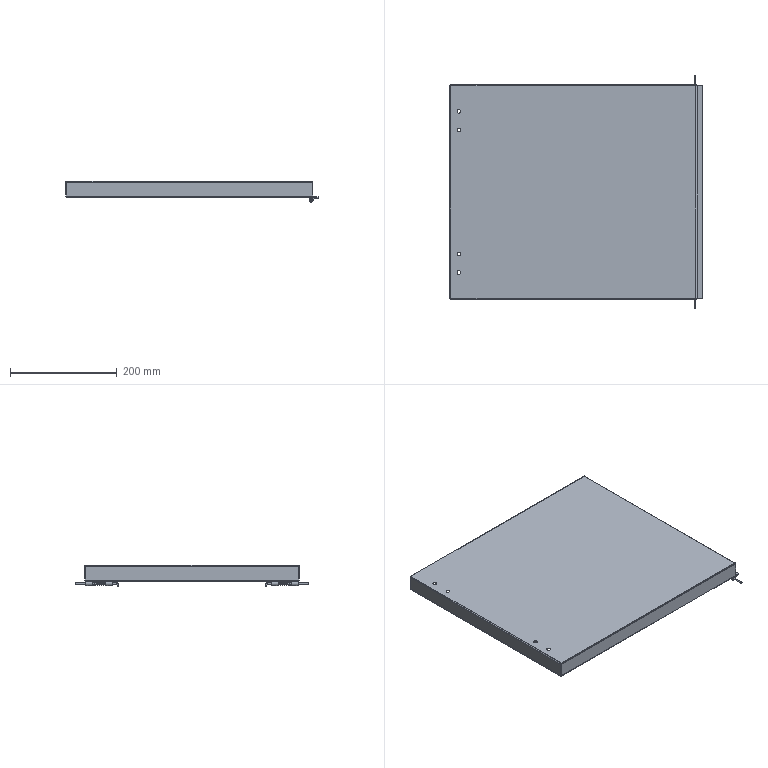Part | 5 solids | 145 faces | box 472.8 x 438.127 x 41 mm | volume 306374 mm3 | plane 76 | cylinder 51 | spline 14 | torus 4 | commonest cylinder face diameters 7 x11 1.473 x8 3 x8 3.6 x8 3.873 x8 7.6 x8